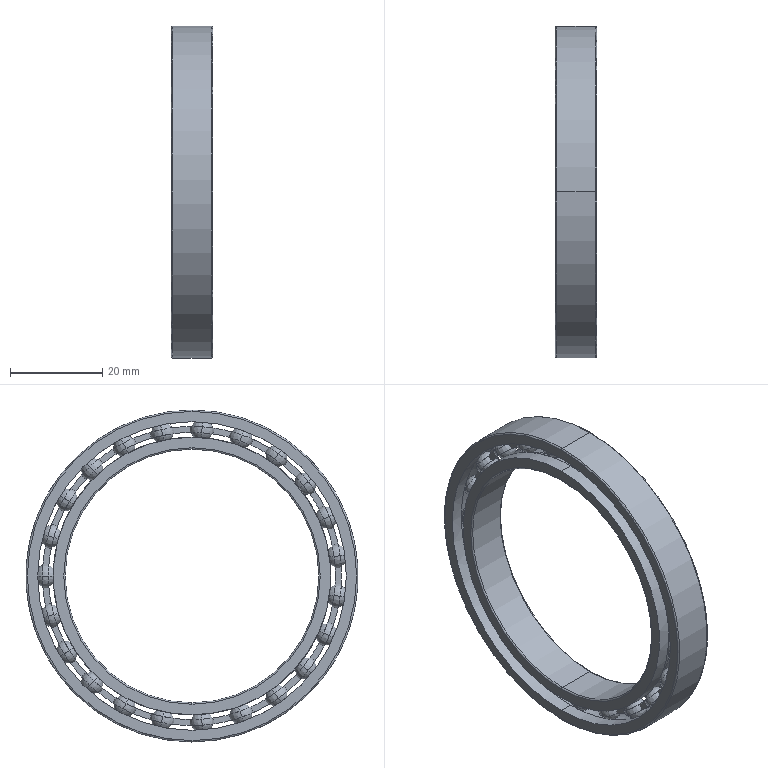Part | SolidWorks | features Revolution 5, CirPattern 2, RevCut 2 | 1 solid | 330 faces | box 9 x 72 x 72 mm | volume 10111 mm3 | sphere 184 | torus 80 | plane 50 | cylinder 16 | commonest cylinder face diameters 60.2 x4 66.9 x4 55 x2 62.24 x2 64.86 x2 72 x2